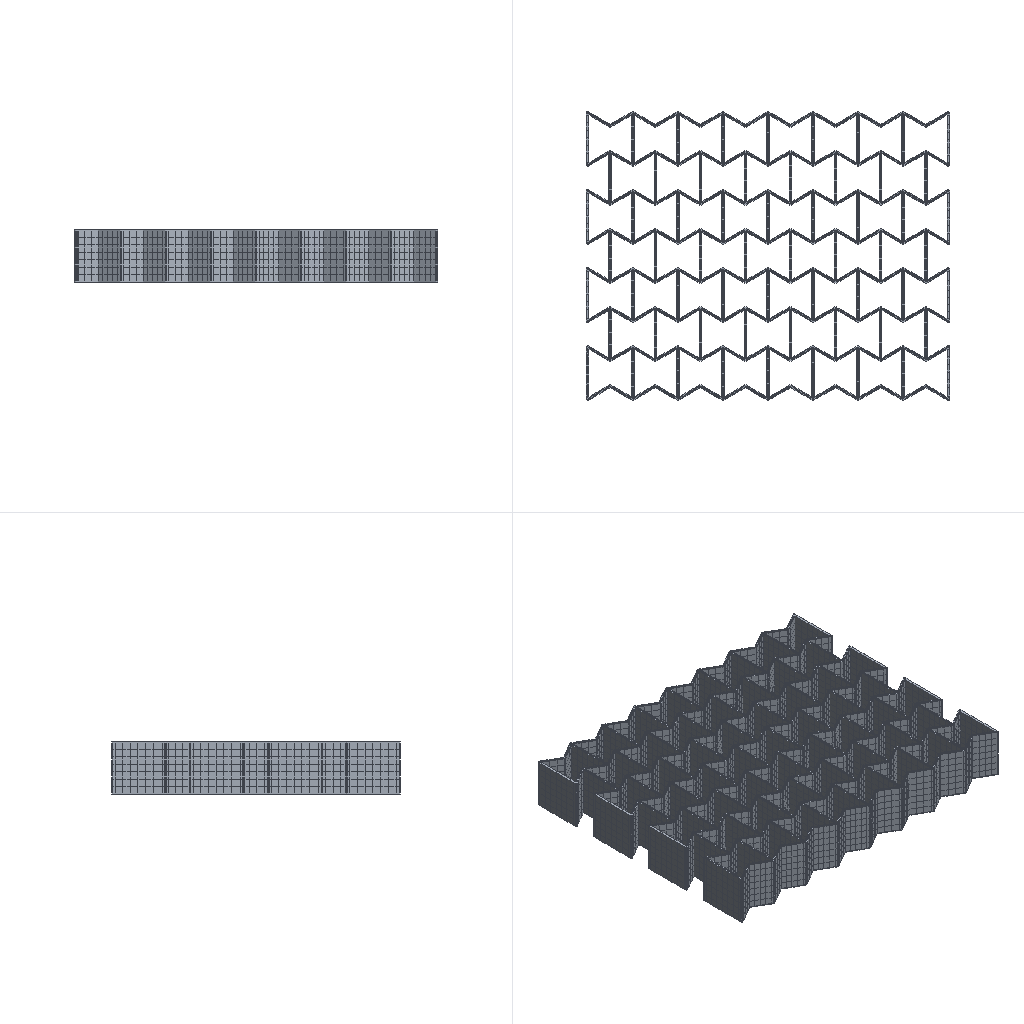Simulation study | abaqus
Set-up summary:
category,name,step,type,value,unit,region
solver,abaqus
solver,version,,,Abaqus/Explicit 2020
units,not stated in the deck,,not stated
analysis,deck,,transient,transient
load_step,Step-1,Step-1,transient
load_step,requested,,,1
mesh,nodes,,,45264
mesh,elements,,,33215
element_type,C3D8R,,solid,33215
load,load commands in deck,,count,1
bc,support commands in deck,,count,7
material,MATERIAL-1,,in results
check,setup vs results,,match,"per instance, exact: element labels, types and connectivity; labels of the nodes the elements use; coordinates of those nodes at SINGLE_PRECISION in 1 of 1 instance(s)"
Abaqus input file, long lists of numbers shortened:
*Heading
** Job name: Job-1 Model name: Model-1
** Generated by: Abaqus/CAE 2020
*Preprint, echo=NO, model=NO, history=NO, contact=NO
**
** PARTS
**
*Part, name=work
*Node
      1,  -73.112,  -31.634,          20.
      2,  -74.112,  -31.634,          20.
** (45262 more lines like these left out)
*Element, type=C3D8R
    1,   990,     3,     2,     1,  6648,  5661,  5660,  5659
    2,   989,   985,     3,   990,  6647,  6643,  5661,  6648
** (33213 more lines like these left out)
*Nset, nset=Set-2, generate
     1,  45264,      1
*Elset, elset=Set-2, generate
     1,  33215,      1
** Section: Section-1
*Solid Section, elset=Set-2, material=Material-1
,
*End Part
**
**
** ASSEMBLY
**
*Assembly, name=Assembly
**
*Instance, name=work-1, part=work
*End Instance
**
*Node
      1,   65.452,         -7.5,          10.
*Nset, nset=Set-1, instance=work-1
     2,     3,     8,    13,    19,    25,    83,    84,   100,   122,   142,   153,   154,   170,   183,   210
   234,   261,   464,   465,   497,   532,   564,   601,  1002,  1003,  1004,  1243,  1244,  1245,  1463,  1464
** (16 more lines like these left out)
*Elset, elset=Set-1, instance=work-1
     1,     6,    28,    29,    30,    31,    47,    69,   323,   403,   490,   492,   494,   496,   618,   653
   714,   763,   925,   926,   927,  1035,  1036,  1151,  2204,  2349,  2518,  2519,  2520,  2521,  2665,  2828
** (12 more lines like these left out)
*Nset, nset=Set-3
 1,
*Nset, nset=m_Set-2
 1,
*Elset, elset=_s_Surf-1_S3, internal, instance=work-1
  3900,  4109,  4583,  4727,  8645,  8854,  9328,  9472, 13390, 13599, 14073, 14217, 18135, 18344, 18818, 18962
 22880, 23089, 23563, 23707, 27625, 27834, 28308, 28452, 32370, 32579, 33053, 33197
*Elset, elset=_s_Surf-1_S6, internal, instance=work-1
  3700,  3852,  3853,  3854,  3855,  4029,  4127,  4128,  4129,  4130,  4386,  4463,  4718,  4728,  4729,  8445
  8597,  8598,  8599,  8600,  8774,  8872,  8873,  8874,  8875,  9131,  9208,  9463,  9473,  9474, 13190, 13342
** (5 more lines like these left out)
*Elset, elset=_s_Surf-1_S4, internal, instance=work-1
  3984,  3985,  4122,  4218,  4526,  4527,  4528,  4529,  4578,  4736,  4743,  4744,  4745,  8729,  8730,  8867
  8963,  9271,  9272,  9273,  9274,  9323,  9481,  9488,  9489,  9490, 13474, 13475, 13612, 13708, 14016, 14017
** (4 more lines like these left out)
*Surface, type=ELEMENT, name=s_Surf-1
_s_Surf-1_S3, S3
_s_Surf-1_S6, S6
_s_Surf-1_S4, S4
** Constraint: Constraint-1
*Coupling, constraint name=Constraint-1, ref node=m_Set-2, surface=s_Surf-1
*Kinematic
*End Assembly
*Amplitude, name=Amp-1
             0.,              0.,            0.01,              1.
**
** MATERIALS
**
*Material, name=Material-1
*Density
 2.7e-09,
*Elastic
72000., 0.28
*Plastic
289.,0.
**
** INTERACTION PROPERTIES
**
*Surface Interaction, name=IntProp-1
*Friction
 0.15,
*Surface Behavior, pressure-overclosure=HARD
** ----------------------------------------------------------------
**
** STEP: Step-1
**
*Step, name=Step-1, nlgeom=YES
*Dynamic, Explicit
, 0.01
*Bulk Viscosity
0.06, 1.2
** Mass Scaling: Semi-Automatic
**               Whole Model
*Fixed Mass Scaling, factor=500.
**
** BOUNDARY CONDITIONS
**
** Name: BC-1 Type: 对称/反对称/完全固定
*Boundary
Set-1, ENCASTRE
** Name: BC-2 Type: 位移/转角
*Boundary, amplitude=Amp-1
Set-3, 1, 1, -70.
Set-3, 2, 2
Set-3, 3, 3
Set-3, 4, 4
Set-3, 5, 5
Set-3, 6, 6
**
** INTERACTIONS
**
** Interaction: Int-1
*Contact, op=NEW
*Contact Inclusions, ALL EXTERIOR
*Contact Property Assignment
 ,  , IntProp-1
**
** OUTPUT REQUESTS
**
*Restart, write, number interval=1, time marks=NO
**
** FIELD OUTPUT: F-Output-1
**
*Output, field, number interval=50
*Node Output
A, CF, RF, RM, RT, U, V
*Element Output, directions=YES
E, EVF, LE, MISES, MISESMAX, PE, PEEQ, PEEQVAVG, PEVAVG, S, SEQUT, SVAVG, YIELDPOT
*Contact Output
CDISP, CSTRESS
**
** HISTORY OUTPUT: H-Output-1
**
*Output, history, time interval=5e-07
*Node Output, nset=Set-3
RF1, U1
*End Step
Results summary:
result,step,Step-1,completed,increments=39546 time=0.01/0.01
result,analysis,,,transient
result,last_loadstep,,,1
result,primary field,,,U
result,reaction total,,FX,-47816.545,model units
result,reaction total,,FY,-1769.289,model units
result,reaction total,,FZ,343.495,model units